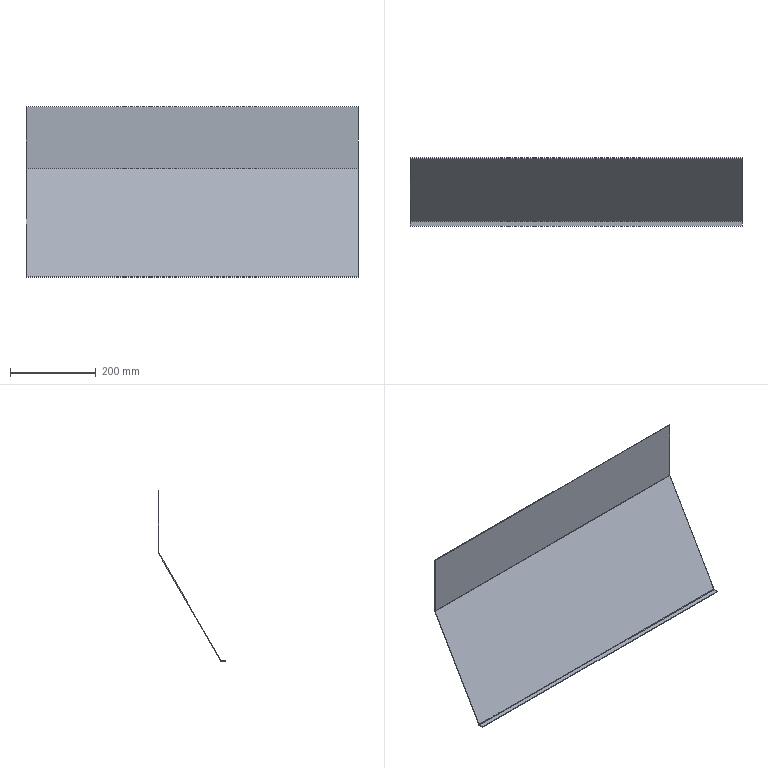Part | NX | features solid 2 | 1 solid | 14 faces | box 776 x 158.714 x 399.116 mm | volume 522508 mm3 | plane 10 | cylinder 4 | commonest cylinder face diameters 3 x2 6 x2
STEP:
#1=CARTESIAN_POINT('',(-332.5,352.853,-601.866));
#2=VERTEX_POINT('',#1);
#3=CARTESIAN_POINT('',(-1108.5,352.853,-601.866));
#4=VERTEX_POINT('',#3);
#5=CARTESIAN_POINT('',(-332.5,352.853,-601.866));
#6=DIRECTION('',(-1.,0.,0.));
#7=VECTOR('',#6,1000.);
#8=LINE('',#5,#7);
#9=EDGE_CURVE('',#2,#4,#8,.T.);
#10=ORIENTED_EDGE('',*,*,#9,.T.);
#11=CARTESIAN_POINT('',(-1108.5,351.554,-602.616));
#12=VERTEX_POINT('',#11);
#13=CARTESIAN_POINT('',(-1108.5,351.554,-601.116));
#14=DIRECTION('',(1.,0.,0.));
#15=DIRECTION('',(0.,1.,0.));
#16=AXIS2_PLACEMENT_3D('',#13,#14,#15);
#17=CIRCLE('',#16,1.5);
#18=EDGE_CURVE('',#12,#4,#17,.T.);
#19=ORIENTED_EDGE('',*,*,#18,.F.);
#20=CARTESIAN_POINT('',(-332.5,351.554,-602.616));
#21=VERTEX_POINT('',#20);
#22=CARTESIAN_POINT('',(-1108.5,351.554,-602.616));
#23=DIRECTION('',(1.,0.,0.));
#24=VECTOR('',#23,1000.);
#25=LINE('',#22,#24);
#26=EDGE_CURVE('',#12,#21,#25,.T.);
#27=ORIENTED_EDGE('',*,*,#26,.T.);
#28=CARTESIAN_POINT('',(-332.5,351.554,-601.116));
#29=DIRECTION('',(1.,0.,0.));
#30=DIRECTION('',(0.,1.,0.));
#31=AXIS2_PLACEMENT_3D('',#28,#29,#30);
#32=CIRCLE('',#31,1.5);
#33=EDGE_CURVE('',#21,#2,#32,.T.);
#34=ORIENTED_EDGE('',*,*,#33,.T.);
#35=EDGE_LOOP('',(#10,#19,#27,#34));
#36=FACE_BOUND('',#35,.T.);
#37=CARTESIAN_POINT('',(-332.5,351.554,-601.116));
#38=DIRECTION('',(-1.,0.,0.));
#39=DIRECTION('',(0.,-0.866,0.5));
#40=AXIS2_PLACEMENT_3D('',#37,#38,#39);
#41=CYLINDRICAL_SURFACE('',#40,1.5);
#42=ADVANCED_FACE('',(#36),#41,.F.);
#43=CARTESIAN_POINT('',(-332.5,354.152,-602.616));
#44=VERTEX_POINT('',#43);
#45=CARTESIAN_POINT('',(-1108.5,354.152,-602.616));
#46=VERTEX_POINT('',#45);
#47=CARTESIAN_POINT('',(-332.5,354.152,-602.616));
#48=DIRECTION('',(-1.,0.,0.));
#49=VECTOR('',#48,1000.);
#50=LINE('',#47,#49);
#51=EDGE_CURVE('',#44,#46,#50,.T.);
#52=ORIENTED_EDGE('',*,*,#51,.F.);
#53=CARTESIAN_POINT('',(-332.5,351.554,-604.116));
#54=VERTEX_POINT('',#53);
#55=CARTESIAN_POINT('',(-332.5,351.554,-601.116));
#56=DIRECTION('',(1.,0.,0.));
#57=DIRECTION('',(0.,-0.866,0.5));
#58=AXIS2_PLACEMENT_3D('',#55,#56,#57);
#59=CIRCLE('',#58,3.);
#60=EDGE_CURVE('',#54,#44,#59,.T.);
#61=ORIENTED_EDGE('',*,*,#60,.F.);
#62=CARTESIAN_POINT('',(-1108.5,351.554,-604.116));
#63=VERTEX_POINT('',#62);
#64=CARTESIAN_POINT('',(-1108.5,351.554,-604.116));
#65=DIRECTION('',(1.,0.,0.));
#66=VECTOR('',#65,1000.);
#67=LINE('',#64,#66);
#68=EDGE_CURVE('',#63,#54,#67,.T.);
#69=ORIENTED_EDGE('',*,*,#68,.F.);
#70=CARTESIAN_POINT('',(-1108.5,351.554,-601.116));
#71=DIRECTION('',(1.,0.,0.));
#72=DIRECTION('',(0.,-0.866,0.5));
#73=AXIS2_PLACEMENT_3D('',#70,#71,#72);
#74=CIRCLE('',#73,3.);
#75=EDGE_CURVE('',#63,#46,#74,.T.);
#76=ORIENTED_EDGE('',*,*,#75,.T.);
#77=EDGE_LOOP('',(#52,#61,#69,#76));
#78=FACE_BOUND('',#77,.T.);
#79=CARTESIAN_POINT('',(-332.5,351.554,-601.116));
#80=DIRECTION('',(-1.,0.,0.));
#81=DIRECTION('',(0.,-0.866,0.5));
#82=AXIS2_PLACEMENT_3D('',#79,#80,#81);
#83=CYLINDRICAL_SURFACE('',#82,3.);
#84=ADVANCED_FACE('',(#78),#83,.T.);
#85=CARTESIAN_POINT('',(-332.5,341.286,-602.616));
#86=VERTEX_POINT('',#85);
#87=CARTESIAN_POINT('',(-1108.5,341.286,-602.616));
#88=VERTEX_POINT('',#87);
#89=CARTESIAN_POINT('',(-332.5,341.286,-602.616));
#90=DIRECTION('',(-1.,0.,0.));
#91=VECTOR('',#90,1000.);
#92=LINE('',#89,#91);
#93=EDGE_CURVE('',#86,#88,#92,.T.);
#94=ORIENTED_EDGE('',*,*,#93,.T.);
#95=CARTESIAN_POINT('',(-1108.5,341.286,-604.116));
#96=VERTEX_POINT('',#95);
#97=CARTESIAN_POINT('',(-1108.5,341.286,-604.116));
#98=DIRECTION('',(0.,0.,1.));
#99=VECTOR('',#98,1000.);
#100=LINE('',#97,#99);
#101=EDGE_CURVE('',#96,#88,#100,.T.);
#102=ORIENTED_EDGE('',*,*,#101,.F.);
#103=CARTESIAN_POINT('',(-332.5,341.286,-604.116));
#104=VERTEX_POINT('',#103);
#105=CARTESIAN_POINT('',(-332.5,341.286,-604.116));
#106=DIRECTION('',(-1.,0.,0.));
#107=VECTOR('',#106,1000.);
#108=LINE('',#105,#107);
#109=EDGE_CURVE('',#104,#96,#108,.T.);
#110=ORIENTED_EDGE('',*,*,#109,.F.);
#111=CARTESIAN_POINT('',(-332.5,341.286,-604.116));
#112=DIRECTION('',(0.,0.,1.));
#113=VECTOR('',#112,1000.);
#114=LINE('',#111,#113);
#115=EDGE_CURVE('',#104,#86,#114,.T.);
#116=ORIENTED_EDGE('',*,*,#115,.T.);
#117=EDGE_LOOP('',(#94,#102,#110,#116));
#118=FACE_BOUND('',#117,.T.);
#119=CARTESIAN_POINT('',(-332.5,341.286,-604.116));
#120=DIRECTION('',(0.,1.,0.));
#121=DIRECTION('',(0.,0.,-1.));
#122=AXIS2_PLACEMENT_3D('',#119,#120,#121);
#123=PLANE('',#122);
#124=ADVANCED_FACE('',(#118),#123,.F.);
#125=ORIENTED_EDGE('',*,*,#26,.F.);
#126=CARTESIAN_POINT('',(-1108.5,352.654,-602.616));
#127=DIRECTION('',(0.,1.,0.));
#128=VECTOR('',#127,1000.);
#129=LINE('',#126,#128);
#130=EDGE_CURVE('',#88,#12,#129,.T.);
#131=ORIENTED_EDGE('',*,*,#130,.F.);
#132=ORIENTED_EDGE('',*,*,#93,.F.);
#133=CARTESIAN_POINT('',(-332.5,352.654,-602.616));
#134=DIRECTION('',(0.,-1.,0.));
#135=VECTOR('',#134,1000.);
#136=LINE('',#133,#135);
#137=EDGE_CURVE('',#21,#86,#136,.T.);
#138=ORIENTED_EDGE('',*,*,#137,.F.);
#139=EDGE_LOOP('',(#125,#131,#132,#138));
#140=FACE_BOUND('',#139,.T.);
#141=CARTESIAN_POINT('',(-722.5,275.,-602.616));
#142=DIRECTION('',(0.,0.,-1.));
#143=DIRECTION('',(-1.,0.,0.));
#144=AXIS2_PLACEMENT_3D('',#141,#142,#143);
#145=PLANE('',#144);
#146=ADVANCED_FACE('',(#140),#145,.F.);
#147=CARTESIAN_POINT('',(-1108.5,352.654,-604.116));
#148=DIRECTION('',(0.,1.,0.));
#149=VECTOR('',#148,1000.);
#150=LINE('',#147,#149);
#151=EDGE_CURVE('',#96,#63,#150,.T.);
#152=ORIENTED_EDGE('',*,*,#151,.T.);
#153=ORIENTED_EDGE('',*,*,#68,.T.);
#154=CARTESIAN_POINT('',(-332.5,352.654,-604.116));
#155=DIRECTION('',(0.,-1.,0.));
#156=VECTOR('',#155,1000.);
#157=LINE('',#154,#156);
#158=EDGE_CURVE('',#54,#104,#157,.T.);
#159=ORIENTED_EDGE('',*,*,#158,.T.);
#160=ORIENTED_EDGE('',*,*,#109,.T.);
#161=EDGE_LOOP('',(#152,#153,#159,#160));
#162=FACE_BOUND('',#161,.T.);
#163=CARTESIAN_POINT('',(-722.5,275.,-604.116));
#164=DIRECTION('',(0.,0.,-1.));
#165=DIRECTION('',(-1.,0.,0.));
#166=AXIS2_PLACEMENT_3D('',#163,#164,#165);
#167=PLANE('',#166);
#168=ADVANCED_FACE('',(#162),#167,.T.);
#169=CARTESIAN_POINT('',(-1108.5,498.5,-349.196));
#170=VERTEX_POINT('',#169);
#171=CARTESIAN_POINT('',(-1108.5,498.5,-205.));
#172=VERTEX_POINT('',#171);
#173=CARTESIAN_POINT('',(-1108.5,498.5,-205.));
#174=DIRECTION('',(0.,0.,1.));
#175=VECTOR('',#174,1000.);
#176=LINE('',#173,#175);
#177=EDGE_CURVE('',#170,#172,#176,.T.);
#178=ORIENTED_EDGE('',*,*,#177,.F.);
#179=CARTESIAN_POINT('',(-332.5,498.5,-349.196));
#180=VERTEX_POINT('',#179);
#181=CARTESIAN_POINT('',(-332.5,498.5,-349.196));
#182=DIRECTION('',(-1.,0.,0.));
#183=VECTOR('',#182,1000.);
#184=LINE('',#181,#183);
#185=EDGE_CURVE('',#180,#170,#184,.T.);
#186=ORIENTED_EDGE('',*,*,#185,.F.);
#187=CARTESIAN_POINT('',(-332.5,498.5,-205.));
#188=VERTEX_POINT('',#187);
#189=CARTESIAN_POINT('',(-332.5,498.5,-205.));
#190=DIRECTION('',(0.,0.,1.));
#191=VECTOR('',#190,1000.);
#192=LINE('',#189,#191);
#193=EDGE_CURVE('',#180,#188,#192,.T.);
#194=ORIENTED_EDGE('',*,*,#193,.T.);
#195=CARTESIAN_POINT('',(-332.5,498.5,-205.));
#196=DIRECTION('',(-1.,0.,0.));
#197=VECTOR('',#196,1000.);
#198=LINE('',#195,#197);
#199=EDGE_CURVE('',#188,#172,#198,.T.);
#200=ORIENTED_EDGE('',*,*,#199,.T.);
#201=EDGE_LOOP('',(#178,#186,#194,#200));
#202=FACE_BOUND('',#201,.T.);
#203=CARTESIAN_POINT('',(-332.5,498.5,-205.));
#204=DIRECTION('',(0.,-1.,0.));
#205=DIRECTION('',(-1.,0.,0.));
#206=AXIS2_PLACEMENT_3D('',#203,#204,#205);
#207=PLANE('',#206);
#208=ADVANCED_FACE('',(#202),#207,.T.);
#209=CARTESIAN_POINT('',(-1108.5,498.299,-349.946));
#210=VERTEX_POINT('',#209);
#211=CARTESIAN_POINT('',(-1108.5,497.,-349.196));
#212=DIRECTION('',(1.,0.,0.));
#213=DIRECTION('',(0.,1.,0.));
#214=AXIS2_PLACEMENT_3D('',#211,#212,#213);
#215=CIRCLE('',#214,1.5);
#216=EDGE_CURVE('',#210,#170,#215,.T.);
#217=ORIENTED_EDGE('',*,*,#216,.F.);
#218=CARTESIAN_POINT('',(-332.5,498.299,-349.946));
#219=VERTEX_POINT('',#218);
#220=CARTESIAN_POINT('',(-332.5,498.299,-349.946));
#221=DIRECTION('',(-1.,0.,0.));
#222=VECTOR('',#221,1000.);
#223=LINE('',#220,#222);
#224=EDGE_CURVE('',#219,#210,#223,.T.);
#225=ORIENTED_EDGE('',*,*,#224,.F.);
#226=CARTESIAN_POINT('',(-332.5,497.,-349.196));
#227=DIRECTION('',(1.,0.,0.));
#228=DIRECTION('',(0.,1.,0.));
#229=AXIS2_PLACEMENT_3D('',#226,#227,#228);
#230=CIRCLE('',#229,1.5);
#231=EDGE_CURVE('',#219,#180,#230,.T.);
#232=ORIENTED_EDGE('',*,*,#231,.T.);
#233=ORIENTED_EDGE('',*,*,#185,.T.);
#234=EDGE_LOOP('',(#217,#225,#232,#233));
#235=FACE_BOUND('',#234,.T.);
#236=CARTESIAN_POINT('',(-332.5,497.,-349.196));
#237=DIRECTION('',(-1.,0.,0.));
#238=DIRECTION('',(0.,1.,0.));
#239=AXIS2_PLACEMENT_3D('',#236,#237,#238);
#240=CYLINDRICAL_SURFACE('',#239,1.5);
#241=ADVANCED_FACE('',(#235),#240,.F.);
#242=ORIENTED_EDGE('',*,*,#9,.F.);
#243=CARTESIAN_POINT('',(-332.5,498.701,-349.25));
#244=DIRECTION('',(0.,0.5,0.866));
#245=VECTOR('',#244,1000.);
#246=LINE('',#243,#245);
#247=EDGE_CURVE('',#2,#219,#246,.T.);
#248=ORIENTED_EDGE('',*,*,#247,.T.);
#249=ORIENTED_EDGE('',*,*,#224,.T.);
#250=CARTESIAN_POINT('',(-1108.5,498.701,-349.25));
#251=DIRECTION('',(0.,0.5,0.866));
#252=VECTOR('',#251,1000.);
#253=LINE('',#250,#252);
#254=EDGE_CURVE('',#4,#210,#253,.T.);
#255=ORIENTED_EDGE('',*,*,#254,.F.);
#256=EDGE_LOOP('',(#242,#248,#249,#255));
#257=FACE_BOUND('',#256,.T.);
#258=CARTESIAN_POINT('',(-332.5,498.701,-349.25));
#259=DIRECTION('',(0.,-0.866,0.5));
#260=DIRECTION('',(-1.,0.,0.));
#261=AXIS2_PLACEMENT_3D('',#258,#259,#260);
#262=PLANE('',#261);
#263=ADVANCED_FACE('',(#257),#262,.T.);
#264=CARTESIAN_POINT('',(-1108.5,500.,-349.196));
#265=VERTEX_POINT('',#264);
#266=CARTESIAN_POINT('',(-1108.5,500.,-205.));
#267=VERTEX_POINT('',#266);
#268=CARTESIAN_POINT('',(-1108.5,500.,-205.));
#269=DIRECTION('',(0.,0.,1.));
#270=VECTOR('',#269,1000.);
#271=LINE('',#268,#270);
#272=EDGE_CURVE('',#265,#267,#271,.T.);
#273=ORIENTED_EDGE('',*,*,#272,.T.);
#274=CARTESIAN_POINT('',(-332.5,500.,-205.));
#275=VERTEX_POINT('',#274);
#276=CARTESIAN_POINT('',(-332.5,500.,-205.));
#277=DIRECTION('',(-1.,0.,0.));
#278=VECTOR('',#277,1000.);
#279=LINE('',#276,#278);
#280=EDGE_CURVE('',#275,#267,#279,.T.);
#281=ORIENTED_EDGE('',*,*,#280,.F.);
#282=CARTESIAN_POINT('',(-332.5,500.,-349.196));
#283=VERTEX_POINT('',#282);
#284=CARTESIAN_POINT('',(-332.5,500.,-205.));
#285=DIRECTION('',(0.,0.,1.));
#286=VECTOR('',#285,1000.);
#287=LINE('',#284,#286);
#288=EDGE_CURVE('',#283,#275,#287,.T.);
#289=ORIENTED_EDGE('',*,*,#288,.F.);
#290=CARTESIAN_POINT('',(-332.5,500.,-349.196));
#291=DIRECTION('',(-1.,0.,0.));
#292=VECTOR('',#291,1000.);
#293=LINE('',#290,#292);
#294=EDGE_CURVE('',#283,#265,#293,.T.);
#295=ORIENTED_EDGE('',*,*,#294,.T.);
#296=EDGE_LOOP('',(#273,#281,#289,#295));
#297=FACE_BOUND('',#296,.T.);
#298=CARTESIAN_POINT('',(-332.5,500.,-205.));
#299=DIRECTION('',(0.,-1.,0.));
#300=DIRECTION('',(-1.,0.,0.));
#301=AXIS2_PLACEMENT_3D('',#298,#299,#300);
#302=PLANE('',#301);
#303=ADVANCED_FACE('',(#297),#302,.F.);
#304=CARTESIAN_POINT('',(-1108.5,499.598,-350.696));
#305=VERTEX_POINT('',#304);
#306=CARTESIAN_POINT('',(-1108.5,497.,-349.196));
#307=DIRECTION('',(1.,0.,0.));
#308=DIRECTION('',(0.,1.,0.));
#309=AXIS2_PLACEMENT_3D('',#306,#307,#308);
#310=CIRCLE('',#309,3.);
#311=EDGE_CURVE('',#305,#265,#310,.T.);
#312=ORIENTED_EDGE('',*,*,#311,.T.);
#313=ORIENTED_EDGE('',*,*,#294,.F.);
#314=CARTESIAN_POINT('',(-332.5,499.598,-350.696));
#315=VERTEX_POINT('',#314);
#316=CARTESIAN_POINT('',(-332.5,497.,-349.196));
#317=DIRECTION('',(1.,0.,0.));
#318=DIRECTION('',(0.,1.,0.));
#319=AXIS2_PLACEMENT_3D('',#316,#317,#318);
#320=CIRCLE('',#319,3.);
#321=EDGE_CURVE('',#315,#283,#320,.T.);
#322=ORIENTED_EDGE('',*,*,#321,.F.);
#323=CARTESIAN_POINT('',(-332.5,499.598,-350.696));
#324=DIRECTION('',(-1.,0.,0.));
#325=VECTOR('',#324,1000.);
#326=LINE('',#323,#325);
#327=EDGE_CURVE('',#315,#305,#326,.T.);
#328=ORIENTED_EDGE('',*,*,#327,.T.);
#329=EDGE_LOOP('',(#312,#313,#322,#328));
#330=FACE_BOUND('',#329,.T.);
#331=CARTESIAN_POINT('',(-332.5,497.,-349.196));
#332=DIRECTION('',(-1.,0.,0.));
#333=DIRECTION('',(0.,1.,0.));
#334=AXIS2_PLACEMENT_3D('',#331,#332,#333);
#335=CYLINDRICAL_SURFACE('',#334,3.);
#336=ADVANCED_FACE('',(#330),#335,.T.);
#337=CARTESIAN_POINT('',(-1108.5,500.,-205.));
#338=DIRECTION('',(0.,1.,0.));
#339=VECTOR('',#338,1000.);
#340=LINE('',#337,#339);
#341=EDGE_CURVE('',#172,#267,#340,.T.);
#342=ORIENTED_EDGE('',*,*,#341,.F.);
#343=ORIENTED_EDGE('',*,*,#199,.F.);
#344=CARTESIAN_POINT('',(-332.5,500.,-205.));
#345=DIRECTION('',(0.,1.,0.));
#346=VECTOR('',#345,1000.);
#347=LINE('',#344,#346);
#348=EDGE_CURVE('',#188,#275,#347,.T.);
#349=ORIENTED_EDGE('',*,*,#348,.T.);
#350=ORIENTED_EDGE('',*,*,#280,.T.);
#351=EDGE_LOOP('',(#342,#343,#349,#350));
#352=FACE_BOUND('',#351,.T.);
#353=CARTESIAN_POINT('',(-332.5,500.,-205.));
#354=DIRECTION('',(0.,0.,1.));
#355=DIRECTION('',(0.,-1.,0.));
#356=AXIS2_PLACEMENT_3D('',#353,#354,#355);
#357=PLANE('',#356);
#358=ADVANCED_FACE('',(#352),#357,.T.);
#359=CARTESIAN_POINT('',(-332.5,500.,-350.));
#360=DIRECTION('',(0.,0.5,0.866));
#361=VECTOR('',#360,1000.);
#362=LINE('',#359,#361);
#363=EDGE_CURVE('',#44,#315,#362,.T.);
#364=ORIENTED_EDGE('',*,*,#363,.F.);
#365=ORIENTED_EDGE('',*,*,#51,.T.);
#366=CARTESIAN_POINT('',(-1108.5,500.,-350.));
#367=DIRECTION('',(0.,0.5,0.866));
#368=VECTOR('',#367,1000.);
#369=LINE('',#366,#368);
#370=EDGE_CURVE('',#46,#305,#369,.T.);
#371=ORIENTED_EDGE('',*,*,#370,.T.);
#372=ORIENTED_EDGE('',*,*,#327,.F.);
#373=EDGE_LOOP('',(#364,#365,#371,#372));
#374=FACE_BOUND('',#373,.T.);
#375=CARTESIAN_POINT('',(-332.5,500.,-350.));
#376=DIRECTION('',(0.,-0.866,0.5));
#377=DIRECTION('',(-1.,0.,0.));
#378=AXIS2_PLACEMENT_3D('',#375,#376,#377);
#379=PLANE('',#378);
#380=ADVANCED_FACE('',(#374),#379,.F.);
#381=ORIENTED_EDGE('',*,*,#370,.F.);
#382=ORIENTED_EDGE('',*,*,#75,.F.);
#383=ORIENTED_EDGE('',*,*,#151,.F.);
#384=ORIENTED_EDGE('',*,*,#101,.T.);
#385=ORIENTED_EDGE('',*,*,#130,.T.);
#386=ORIENTED_EDGE('',*,*,#18,.T.);
#387=ORIENTED_EDGE('',*,*,#254,.T.);
#388=ORIENTED_EDGE('',*,*,#216,.T.);
#389=ORIENTED_EDGE('',*,*,#177,.T.);
#390=ORIENTED_EDGE('',*,*,#341,.T.);
#391=ORIENTED_EDGE('',*,*,#272,.F.);
#392=ORIENTED_EDGE('',*,*,#311,.F.);
#393=EDGE_LOOP('',(#381,#382,#383,#384,#385,#386,#387,#388,#389,#390,#391,#392));
#394=FACE_BOUND('',#393,.T.);
#395=CARTESIAN_POINT('',(-1108.5,497.,-349.196));
#396=DIRECTION('',(1.,0.,0.));
#397=DIRECTION('',(0.,-1.,0.));
#398=AXIS2_PLACEMENT_3D('',#395,#396,#397);
#399=PLANE('',#398);
#400=ADVANCED_FACE('',(#394),#399,.F.);
#401=ORIENTED_EDGE('',*,*,#247,.F.);
#402=ORIENTED_EDGE('',*,*,#33,.F.);
#403=ORIENTED_EDGE('',*,*,#137,.T.);
#404=ORIENTED_EDGE('',*,*,#115,.F.);
#405=ORIENTED_EDGE('',*,*,#158,.F.);
#406=ORIENTED_EDGE('',*,*,#60,.T.);
#407=ORIENTED_EDGE('',*,*,#363,.T.);
#408=ORIENTED_EDGE('',*,*,#321,.T.);
#409=ORIENTED_EDGE('',*,*,#288,.T.);
#410=ORIENTED_EDGE('',*,*,#348,.F.);
#411=ORIENTED_EDGE('',*,*,#193,.F.);
#412=ORIENTED_EDGE('',*,*,#231,.F.);
#413=EDGE_LOOP('',(#401,#402,#403,#404,#405,#406,#407,#408,#409,#410,#411,#412));
#414=FACE_BOUND('',#413,.T.);
#415=CARTESIAN_POINT('',(-332.5,500.,-350.));
#416=DIRECTION('',(1.,0.,0.));
#417=DIRECTION('',(0.,-1.,0.));
#418=AXIS2_PLACEMENT_3D('',#415,#416,#417);
#419=PLANE('',#418);
#420=ADVANCED_FACE('',(#414),#419,.T.);
#421=CLOSED_SHELL('',(#42,#84,#124,#146,#168,#208,#241,#263,#303,#336,#358,#380,#400,#420));
#422=MANIFOLD_SOLID_BREP('',#421);
#423=(LENGTH_UNIT()NAMED_UNIT(*)SI_UNIT(.MILLI.,.METRE.));
#424=UNCERTAINTY_MEASURE_WITH_UNIT(LENGTH_MEASURE(0.00001),#423,'','');
#425=(NAMED_UNIT(*)PLANE_ANGLE_UNIT()SI_UNIT($,.RADIAN.));
#426=(NAMED_UNIT(*)SI_UNIT($,.STERADIAN.)SOLID_ANGLE_UNIT());
#427=(GEOMETRIC_REPRESENTATION_CONTEXT(3)GLOBAL_UNCERTAINTY_ASSIGNED_CONTEXT((#424))GLOBAL_UNIT_ASSIGNED_CONTEXT((#423,#425,#426))REPRESENTATION_CONTEXT('',''));
#428=ADVANCED_BREP_SHAPE_REPRESENTATION('',(#422),#427);